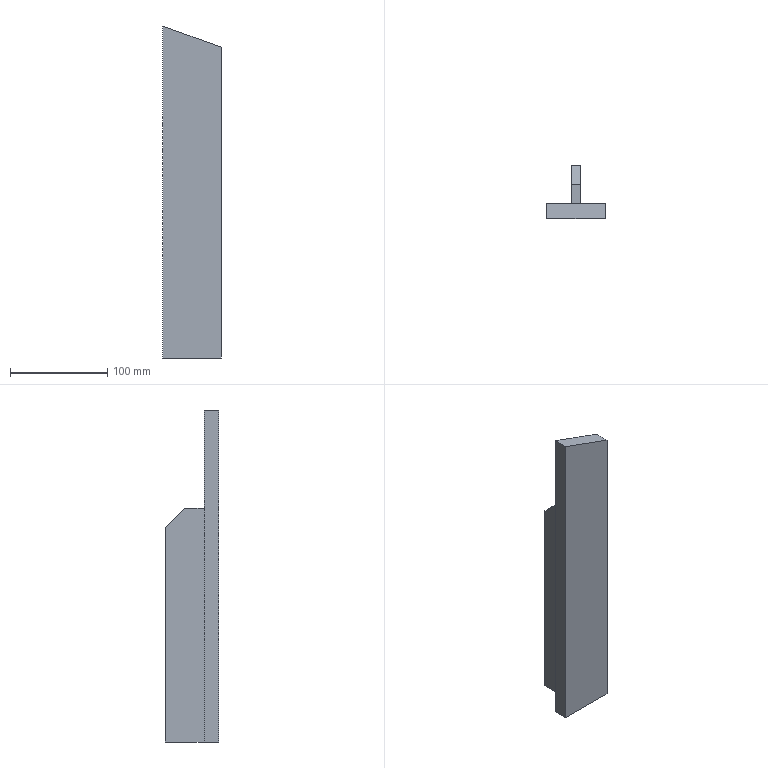Part | NX | features solid 2 | 1 solid | 11 faces | box 60 x 55 x 340.764 mm | volume 390861 mm3 | plane 11
STEP:
#1=CARTESIAN_POINT('',(-745.,-827.5,-270.));
#2=VERTEX_POINT('',#1);
#3=CARTESIAN_POINT('',(-745.,-842.5,-270.));
#4=VERTEX_POINT('',#3);
#5=CARTESIAN_POINT('',(-745.,-835.,-270.));
#6=DIRECTION('',(0.,1.,0.));
#7=VECTOR('',#6,1000.);
#8=LINE('',#5,#7);
#9=EDGE_CURVE('',#2,#4,#8,.F.);
#10=ORIENTED_EDGE('',*,*,#9,.F.);
#11=CARTESIAN_POINT('',(-720.,-827.5,-270.));
#12=VERTEX_POINT('',#11);
#13=CARTESIAN_POINT('',(-745.,-827.5,-270.));
#14=DIRECTION('',(1.,0.,0.));
#15=VECTOR('',#14,1000.);
#16=LINE('',#13,#15);
#17=EDGE_CURVE('',#2,#12,#16,.T.);
#18=ORIENTED_EDGE('',*,*,#17,.T.);
#19=CARTESIAN_POINT('',(-720.,-787.5,-270.));
#20=VERTEX_POINT('',#19);
#21=CARTESIAN_POINT('',(-720.,-827.5,-270.));
#22=DIRECTION('',(0.,1.,0.));
#23=VECTOR('',#22,1000.);
#24=LINE('',#21,#23);
#25=EDGE_CURVE('',#12,#20,#24,.T.);
#26=ORIENTED_EDGE('',*,*,#25,.T.);
#27=CARTESIAN_POINT('',(-710.,-787.5,-270.));
#28=VERTEX_POINT('',#27);
#29=CARTESIAN_POINT('',(-745.,-787.5,-270.));
#30=DIRECTION('',(1.,0.,0.));
#31=VECTOR('',#30,1000.);
#32=LINE('',#29,#31);
#33=EDGE_CURVE('',#20,#28,#32,.T.);
#34=ORIENTED_EDGE('',*,*,#33,.T.);
#35=CARTESIAN_POINT('',(-710.,-827.5,-270.));
#36=VERTEX_POINT('',#35);
#37=CARTESIAN_POINT('',(-710.,-827.5,-270.));
#38=DIRECTION('',(0.,1.,0.));
#39=VECTOR('',#38,1000.);
#40=LINE('',#37,#39);
#41=EDGE_CURVE('',#36,#28,#40,.T.);
#42=ORIENTED_EDGE('',*,*,#41,.F.);
#43=CARTESIAN_POINT('',(-685.,-827.5,-270.));
#44=VERTEX_POINT('',#43);
#45=CARTESIAN_POINT('',(-745.,-827.5,-270.));
#46=DIRECTION('',(1.,0.,0.));
#47=VECTOR('',#46,1000.);
#48=LINE('',#45,#47);
#49=EDGE_CURVE('',#36,#44,#48,.T.);
#50=ORIENTED_EDGE('',*,*,#49,.T.);
#51=CARTESIAN_POINT('',(-685.,-842.5,-270.));
#52=VERTEX_POINT('',#51);
#53=CARTESIAN_POINT('',(-685.,-835.,-270.));
#54=DIRECTION('',(0.,1.,0.));
#55=VECTOR('',#54,1000.);
#56=LINE('',#53,#55);
#57=EDGE_CURVE('',#44,#52,#56,.F.);
#58=ORIENTED_EDGE('',*,*,#57,.T.);
#59=CARTESIAN_POINT('',(-745.,-842.5,-270.));
#60=DIRECTION('',(1.,0.,0.));
#61=VECTOR('',#60,1000.);
#62=LINE('',#59,#61);
#63=EDGE_CURVE('',#4,#52,#62,.T.);
#64=ORIENTED_EDGE('',*,*,#63,.F.);
#65=EDGE_LOOP('',(#10,#18,#26,#34,#42,#50,#58,#64));
#66=FACE_BOUND('',#65,.T.);
#67=CARTESIAN_POINT('',(-685.,-842.5,-270.));
#68=DIRECTION('',(0.,0.,-1.));
#69=DIRECTION('',(-1.,0.,0.));
#70=AXIS2_PLACEMENT_3D('',#67,#68,#69);
#71=PLANE('',#70);
#72=ADVANCED_FACE('',(#66),#71,.T.);
#73=CARTESIAN_POINT('',(-720.,-807.5,-30.));
#74=VERTEX_POINT('',#73);
#75=CARTESIAN_POINT('',(-720.,-787.5,-50.));
#76=VERTEX_POINT('',#75);
#77=CARTESIAN_POINT('',(-720.,-787.5,-50.));
#78=DIRECTION('',(0.,0.7071,-0.7071));
#79=VECTOR('',#78,1000.);
#80=LINE('',#77,#79);
#81=EDGE_CURVE('',#74,#76,#80,.T.);
#82=ORIENTED_EDGE('',*,*,#81,.F.);
#83=CARTESIAN_POINT('',(-710.,-807.5,-30.));
#84=VERTEX_POINT('',#83);
#85=CARTESIAN_POINT('',(-715.,-807.5,-30.));
#86=DIRECTION('',(1.,0.,0.));
#87=VECTOR('',#86,1000.);
#88=LINE('',#85,#87);
#89=EDGE_CURVE('',#84,#74,#88,.F.);
#90=ORIENTED_EDGE('',*,*,#89,.F.);
#91=CARTESIAN_POINT('',(-710.,-787.5,-50.));
#92=VERTEX_POINT('',#91);
#93=CARTESIAN_POINT('',(-710.,-717.5,-120.));
#94=DIRECTION('',(0.,-0.7071,0.7071));
#95=VECTOR('',#94,1000.);
#96=LINE('',#93,#95);
#97=EDGE_CURVE('',#92,#84,#96,.T.);
#98=ORIENTED_EDGE('',*,*,#97,.F.);
#99=CARTESIAN_POINT('',(-715.,-787.5,-50.));
#100=DIRECTION('',(1.,0.,0.));
#101=VECTOR('',#100,1000.);
#102=LINE('',#99,#101);
#103=EDGE_CURVE('',#76,#92,#102,.T.);
#104=ORIENTED_EDGE('',*,*,#103,.F.);
#105=EDGE_LOOP('',(#82,#90,#98,#104));
#106=FACE_BOUND('',#105,.T.);
#107=CARTESIAN_POINT('',(-715.,-787.5,-50.));
#108=DIRECTION('',(0.,0.7071,0.7071));
#109=DIRECTION('',(0.,-0.7071,0.7071));
#110=AXIS2_PLACEMENT_3D('',#107,#108,#109);
#111=PLANE('',#110);
#112=ADVANCED_FACE('',(#106),#111,.T.);
#113=CARTESIAN_POINT('',(-710.,-827.5,-30.));
#114=VERTEX_POINT('',#113);
#115=CARTESIAN_POINT('',(-710.,-827.5,-30.));
#116=DIRECTION('',(0.,1.,0.));
#117=VECTOR('',#116,1000.);
#118=LINE('',#115,#117);
#119=EDGE_CURVE('',#114,#84,#118,.T.);
#120=ORIENTED_EDGE('',*,*,#119,.T.);
#121=ORIENTED_EDGE('',*,*,#89,.T.);
#122=CARTESIAN_POINT('',(-720.,-827.5,-30.));
#123=VERTEX_POINT('',#122);
#124=CARTESIAN_POINT('',(-720.,-827.5,-30.));
#125=DIRECTION('',(0.,1.,0.));
#126=VECTOR('',#125,1000.);
#127=LINE('',#124,#126);
#128=EDGE_CURVE('',#123,#74,#127,.T.);
#129=ORIENTED_EDGE('',*,*,#128,.F.);
#130=CARTESIAN_POINT('',(-715.,-827.5,-30.));
#131=DIRECTION('',(1.,0.,0.));
#132=VECTOR('',#131,1000.);
#133=LINE('',#130,#132);
#134=EDGE_CURVE('',#123,#114,#133,.T.);
#135=ORIENTED_EDGE('',*,*,#134,.T.);
#136=EDGE_LOOP('',(#120,#121,#129,#135));
#137=FACE_BOUND('',#136,.T.);
#138=CARTESIAN_POINT('',(-715.,-827.5,-30.));
#139=DIRECTION('',(0.,0.,-1.));
#140=DIRECTION('',(0.,1.,0.));
#141=AXIS2_PLACEMENT_3D('',#138,#139,#140);
#142=PLANE('',#141);
#143=ADVANCED_FACE('',(#137),#142,.F.);
#144=CARTESIAN_POINT('',(-685.,-827.5,48.926));
#145=VERTEX_POINT('',#144);
#146=CARTESIAN_POINT('',(-685.,-842.5,48.926));
#147=VERTEX_POINT('',#146);
#148=CARTESIAN_POINT('',(-685.,-835.,48.926));
#149=DIRECTION('',(0.,1.,0.));
#150=VECTOR('',#149,1000.);
#151=LINE('',#148,#150);
#152=EDGE_CURVE('',#145,#147,#151,.F.);
#153=ORIENTED_EDGE('',*,*,#152,.F.);
#154=CARTESIAN_POINT('',(-745.,-827.5,70.764));
#155=VERTEX_POINT('',#154);
#156=CARTESIAN_POINT('',(-704.72,-827.5,56.104));
#157=DIRECTION('',(0.9397,0.,-0.342));
#158=VECTOR('',#157,1000.);
#159=LINE('',#156,#158);
#160=EDGE_CURVE('',#155,#145,#159,.T.);
#161=ORIENTED_EDGE('',*,*,#160,.F.);
#162=CARTESIAN_POINT('',(-745.,-842.5,70.764));
#163=VERTEX_POINT('',#162);
#164=CARTESIAN_POINT('',(-745.,-885.,70.764));
#165=DIRECTION('',(0.,-1.,0.));
#166=VECTOR('',#165,1000.);
#167=LINE('',#164,#166);
#168=EDGE_CURVE('',#163,#155,#167,.F.);
#169=ORIENTED_EDGE('',*,*,#168,.F.);
#170=CARTESIAN_POINT('',(-737.38,-842.5,67.991));
#171=DIRECTION('',(-0.9397,0.,0.342));
#172=VECTOR('',#171,1000.);
#173=LINE('',#170,#172);
#174=EDGE_CURVE('',#147,#163,#173,.T.);
#175=ORIENTED_EDGE('',*,*,#174,.F.);
#176=EDGE_LOOP('',(#153,#161,#169,#175));
#177=FACE_BOUND('',#176,.T.);
#178=CARTESIAN_POINT('',(-704.72,-885.,56.104));
#179=DIRECTION('',(-0.342,0.,-0.9397));
#180=DIRECTION('',(-0.9397,0.,0.342));
#181=AXIS2_PLACEMENT_3D('',#178,#179,#180);
#182=PLANE('',#181);
#183=ADVANCED_FACE('',(#177),#182,.F.);
#184=ORIENTED_EDGE('',*,*,#128,.T.);
#185=ORIENTED_EDGE('',*,*,#81,.T.);
#186=CARTESIAN_POINT('',(-720.,-787.5,-230.));
#187=DIRECTION('',(0.,0.,1.));
#188=VECTOR('',#187,1000.);
#189=LINE('',#186,#188);
#190=EDGE_CURVE('',#20,#76,#189,.T.);
#191=ORIENTED_EDGE('',*,*,#190,.F.);
#192=ORIENTED_EDGE('',*,*,#25,.F.);
#193=CARTESIAN_POINT('',(-720.,-827.5,-230.));
#194=DIRECTION('',(0.,0.,1.));
#195=VECTOR('',#194,1000.);
#196=LINE('',#193,#195);
#197=EDGE_CURVE('',#12,#123,#196,.T.);
#198=ORIENTED_EDGE('',*,*,#197,.T.);
#199=EDGE_LOOP('',(#184,#185,#191,#192,#198));
#200=FACE_BOUND('',#199,.T.);
#201=CARTESIAN_POINT('',(-720.,-827.5,-230.));
#202=DIRECTION('',(1.,0.,0.));
#203=DIRECTION('',(0.,1.,0.));
#204=AXIS2_PLACEMENT_3D('',#201,#202,#203);
#205=PLANE('',#204);
#206=ADVANCED_FACE('',(#200),#205,.F.);
#207=ORIENTED_EDGE('',*,*,#190,.T.);
#208=ORIENTED_EDGE('',*,*,#103,.T.);
#209=CARTESIAN_POINT('',(-710.,-787.5,-230.));
#210=DIRECTION('',(0.,0.,1.));
#211=VECTOR('',#210,1000.);
#212=LINE('',#209,#211);
#213=EDGE_CURVE('',#28,#92,#212,.T.);
#214=ORIENTED_EDGE('',*,*,#213,.F.);
#215=ORIENTED_EDGE('',*,*,#33,.F.);
#216=EDGE_LOOP('',(#207,#208,#214,#215));
#217=FACE_BOUND('',#216,.T.);
#218=CARTESIAN_POINT('',(-715.,-787.5,-230.));
#219=DIRECTION('',(0.,1.,0.));
#220=DIRECTION('',(0.,0.,1.));
#221=AXIS2_PLACEMENT_3D('',#218,#219,#220);
#222=PLANE('',#221);
#223=ADVANCED_FACE('',(#217),#222,.T.);
#224=ORIENTED_EDGE('',*,*,#213,.T.);
#225=ORIENTED_EDGE('',*,*,#97,.T.);
#226=ORIENTED_EDGE('',*,*,#119,.F.);
#227=CARTESIAN_POINT('',(-710.,-827.5,-230.));
#228=DIRECTION('',(0.,0.,1.));
#229=VECTOR('',#228,1000.);
#230=LINE('',#227,#229);
#231=EDGE_CURVE('',#36,#114,#230,.T.);
#232=ORIENTED_EDGE('',*,*,#231,.F.);
#233=ORIENTED_EDGE('',*,*,#41,.T.);
#234=EDGE_LOOP('',(#224,#225,#226,#232,#233));
#235=FACE_BOUND('',#234,.T.);
#236=CARTESIAN_POINT('',(-710.,-827.5,-230.));
#237=DIRECTION('',(1.,0.,0.));
#238=DIRECTION('',(0.,1.,0.));
#239=AXIS2_PLACEMENT_3D('',#236,#237,#238);
#240=PLANE('',#239);
#241=ADVANCED_FACE('',(#235),#240,.T.);
#242=CARTESIAN_POINT('',(-685.,-827.5,28.621));
#243=DIRECTION('',(0.,0.,1.));
#244=VECTOR('',#243,1000.);
#245=LINE('',#242,#244);
#246=EDGE_CURVE('',#145,#44,#245,.F.);
#247=ORIENTED_EDGE('',*,*,#246,.F.);
#248=ORIENTED_EDGE('',*,*,#152,.T.);
#249=CARTESIAN_POINT('',(-685.,-842.5,28.621));
#250=DIRECTION('',(0.,0.,1.));
#251=VECTOR('',#250,1000.);
#252=LINE('',#249,#251);
#253=EDGE_CURVE('',#147,#52,#252,.F.);
#254=ORIENTED_EDGE('',*,*,#253,.T.);
#255=ORIENTED_EDGE('',*,*,#57,.F.);
#256=EDGE_LOOP('',(#247,#248,#254,#255));
#257=FACE_BOUND('',#256,.T.);
#258=CARTESIAN_POINT('',(-685.,-835.,28.621));
#259=DIRECTION('',(1.,0.,0.));
#260=DIRECTION('',(0.,0.,-1.));
#261=AXIS2_PLACEMENT_3D('',#258,#259,#260);
#262=PLANE('',#261);
#263=ADVANCED_FACE('',(#257),#262,.T.);
#264=ORIENTED_EDGE('',*,*,#253,.F.);
#265=ORIENTED_EDGE('',*,*,#174,.T.);
#266=CARTESIAN_POINT('',(-745.,-842.5,58.205));
#267=DIRECTION('',(0.,0.,-1.));
#268=VECTOR('',#267,1000.);
#269=LINE('',#266,#268);
#270=EDGE_CURVE('',#163,#4,#269,.T.);
#271=ORIENTED_EDGE('',*,*,#270,.T.);
#272=ORIENTED_EDGE('',*,*,#63,.T.);
#273=EDGE_LOOP('',(#264,#265,#271,#272));
#274=FACE_BOUND('',#273,.T.);
#275=CARTESIAN_POINT('',(-740.942,-842.5,58.205));
#276=DIRECTION('',(0.,1.,0.));
#277=DIRECTION('',(-1.,0.,0.));
#278=AXIS2_PLACEMENT_3D('',#275,#276,#277);
#279=PLANE('',#278);
#280=ADVANCED_FACE('',(#274),#279,.F.);
#281=ORIENTED_EDGE('',*,*,#160,.T.);
#282=ORIENTED_EDGE('',*,*,#246,.T.);
#283=ORIENTED_EDGE('',*,*,#49,.F.);
#284=ORIENTED_EDGE('',*,*,#231,.T.);
#285=ORIENTED_EDGE('',*,*,#134,.F.);
#286=ORIENTED_EDGE('',*,*,#197,.F.);
#287=ORIENTED_EDGE('',*,*,#17,.F.);
#288=CARTESIAN_POINT('',(-745.,-827.5,58.205));
#289=DIRECTION('',(0.,0.,-1.));
#290=VECTOR('',#289,1000.);
#291=LINE('',#288,#290);
#292=EDGE_CURVE('',#155,#2,#291,.T.);
#293=ORIENTED_EDGE('',*,*,#292,.F.);
#294=EDGE_LOOP('',(#281,#282,#283,#284,#285,#286,#287,#293));
#295=FACE_BOUND('',#294,.T.);
#296=CARTESIAN_POINT('',(-740.942,-827.5,58.205));
#297=DIRECTION('',(0.,1.,0.));
#298=DIRECTION('',(-1.,0.,0.));
#299=AXIS2_PLACEMENT_3D('',#296,#297,#298);
#300=PLANE('',#299);
#301=ADVANCED_FACE('',(#295),#300,.T.);
#302=ORIENTED_EDGE('',*,*,#292,.T.);
#303=ORIENTED_EDGE('',*,*,#9,.T.);
#304=ORIENTED_EDGE('',*,*,#270,.F.);
#305=ORIENTED_EDGE('',*,*,#168,.T.);
#306=EDGE_LOOP('',(#302,#303,#304,#305));
#307=FACE_BOUND('',#306,.T.);
#308=CARTESIAN_POINT('',(-745.,-835.,58.205));
#309=DIRECTION('',(1.,0.,0.));
#310=DIRECTION('',(0.,0.,-1.));
#311=AXIS2_PLACEMENT_3D('',#308,#309,#310);
#312=PLANE('',#311);
#313=ADVANCED_FACE('',(#307),#312,.F.);
#314=CLOSED_SHELL('',(#72,#112,#143,#183,#206,#223,#241,#263,#280,#301,#313));
#315=MANIFOLD_SOLID_BREP('',#314);
#316=(LENGTH_UNIT()NAMED_UNIT(*)SI_UNIT(.MILLI.,.METRE.));
#317=UNCERTAINTY_MEASURE_WITH_UNIT(LENGTH_MEASURE(0.00001),#316,'','');
#318=(NAMED_UNIT(*)PLANE_ANGLE_UNIT()SI_UNIT($,.RADIAN.));
#319=(NAMED_UNIT(*)SI_UNIT($,.STERADIAN.)SOLID_ANGLE_UNIT());
#320=(GEOMETRIC_REPRESENTATION_CONTEXT(3)GLOBAL_UNCERTAINTY_ASSIGNED_CONTEXT((#317))GLOBAL_UNIT_ASSIGNED_CONTEXT((#316,#318,#319))REPRESENTATION_CONTEXT('',''));
#321=ADVANCED_BREP_SHAPE_REPRESENTATION('',(#315),#320);